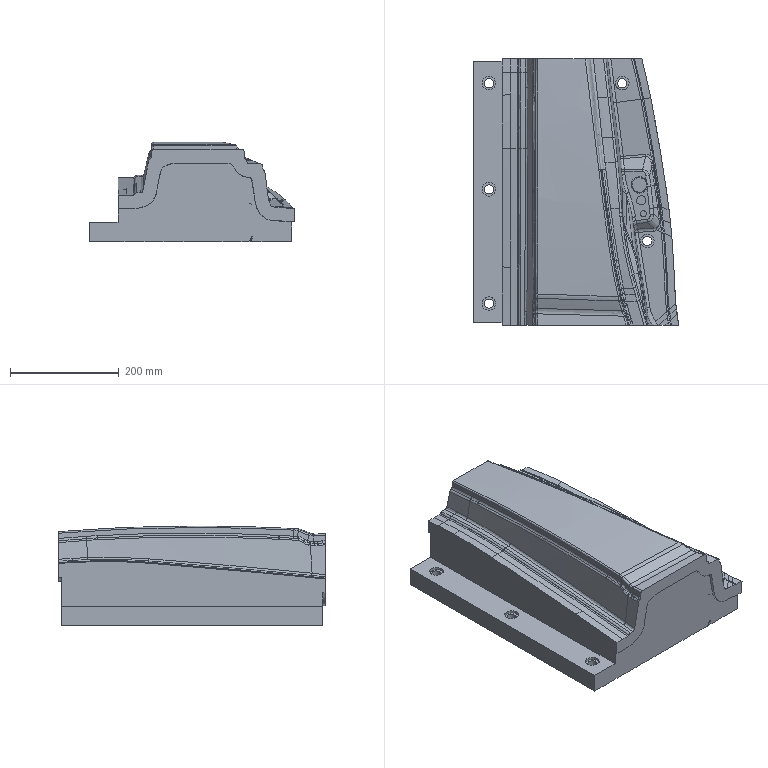Part | NX | features solid 2 | 1 solid | 358 faces | box 377.974 x 490 x 182.843 mm | volume 15256060 mm3 | spline 223 | cylinder 89 | plane 42 | cone 4 | commonest cylinder face diameters 6 x8 10 x6 6.001 x5 6.004 x5 17 x5 20 x5